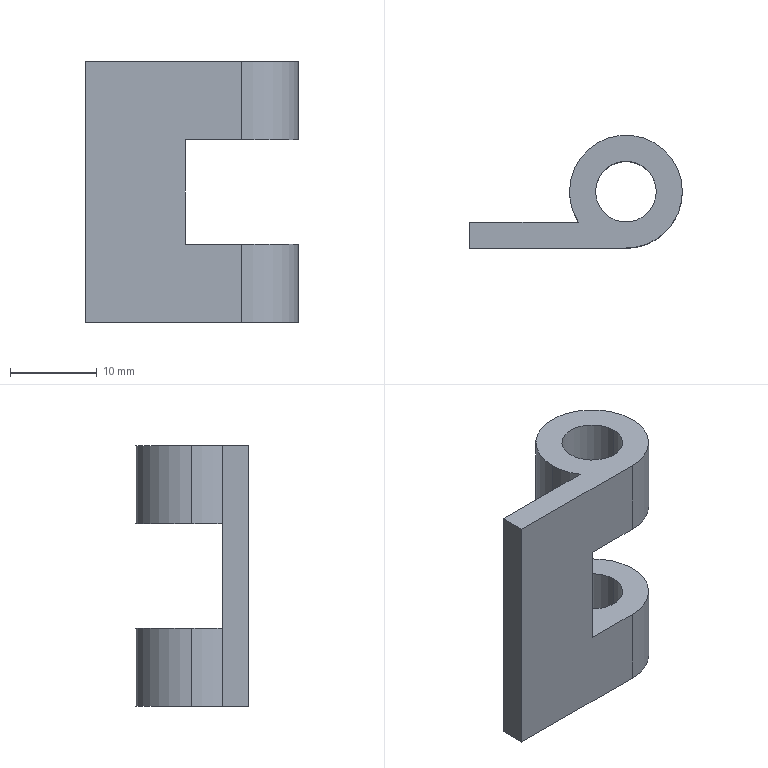Part | SolidWorks | features Extrusion 1, ICE 1 | 1 solid | 18 faces | box 24.5 x 13 x 30 mm | volume 2874 mm3 | cylinder 10 | plane 8 | commonest cylinder face diameters 13 x6 7 x4
STEP:
#1=CARTESIAN_POINT('',(5.5,5.,30.));
#2=VERTEX_POINT('',#1);
#3=CARTESIAN_POINT('',(12.5,5.,30.));
#4=VERTEX_POINT('',#3);
#5=CARTESIAN_POINT('',(9.,5.,30.));
#6=DIRECTION('',(0.,0.,1.));
#7=DIRECTION('',(1.,0.,0.));
#8=AXIS2_PLACEMENT_3D('',#5,#6,#7);
#9=CIRCLE('',#8,3.5);
#10=EDGE_CURVE('',#2,#4,#9,.T.);
#11=ORIENTED_EDGE('',*,*,#10,.T.);
#12=CARTESIAN_POINT('',(12.5,5.,21.));
#13=VERTEX_POINT('',#12);
#14=CARTESIAN_POINT('',(12.5,5.,30.));
#15=DIRECTION('',(0.,0.,-1.));
#16=VECTOR('',#15,1000.);
#17=LINE('',#14,#16);
#18=EDGE_CURVE('',#4,#13,#17,.T.);
#19=ORIENTED_EDGE('',*,*,#18,.T.);
#20=CARTESIAN_POINT('',(5.5,5.,21.));
#21=VERTEX_POINT('',#20);
#22=CARTESIAN_POINT('',(9.,5.,21.));
#23=DIRECTION('',(0.,0.,1.));
#24=DIRECTION('',(1.,0.,0.));
#25=AXIS2_PLACEMENT_3D('',#22,#23,#24);
#26=CIRCLE('',#25,3.5);
#27=EDGE_CURVE('',#21,#13,#26,.T.);
#28=ORIENTED_EDGE('',*,*,#27,.F.);
#29=CARTESIAN_POINT('',(5.5,5.,30.));
#30=DIRECTION('',(0.,0.,-1.));
#31=VECTOR('',#30,1000.);
#32=LINE('',#29,#31);
#33=EDGE_CURVE('',#2,#21,#32,.T.);
#34=ORIENTED_EDGE('',*,*,#33,.F.);
#35=EDGE_LOOP('',(#11,#19,#28,#34));
#36=FACE_OUTER_BOUND('',#35,.T.);
#37=CARTESIAN_POINT('',(9.,5.,30.));
#38=DIRECTION('',(0.,0.,-1.));
#39=DIRECTION('',(-1.,0.,0.));
#40=AXIS2_PLACEMENT_3D('',#37,#38,#39);
#41=CYLINDRICAL_SURFACE('',#40,3.5);
#42=ADVANCED_FACE('',(#36),#41,.F.);
#43=CARTESIAN_POINT('',(15.5,5.,30.));
#44=VERTEX_POINT('',#43);
#45=CARTESIAN_POINT('',(2.5,5.,30.));
#46=VERTEX_POINT('',#45);
#47=CARTESIAN_POINT('',(9.,5.,30.));
#48=DIRECTION('',(0.,0.,1.));
#49=DIRECTION('',(1.,0.,0.));
#50=AXIS2_PLACEMENT_3D('',#47,#48,#49);
#51=CIRCLE('',#50,6.5);
#52=EDGE_CURVE('',#44,#46,#51,.T.);
#53=ORIENTED_EDGE('',*,*,#52,.F.);
#54=CARTESIAN_POINT('',(15.5,5.,21.));
#55=VERTEX_POINT('',#54);
#56=CARTESIAN_POINT('',(15.5,5.,30.));
#57=DIRECTION('',(0.,0.,-1.));
#58=VECTOR('',#57,1000.);
#59=LINE('',#56,#58);
#60=EDGE_CURVE('',#44,#55,#59,.T.);
#61=ORIENTED_EDGE('',*,*,#60,.T.);
#62=CARTESIAN_POINT('',(2.5,5.,21.));
#63=VERTEX_POINT('',#62);
#64=CARTESIAN_POINT('',(9.,5.,21.));
#65=DIRECTION('',(0.,0.,1.));
#66=DIRECTION('',(1.,0.,0.));
#67=AXIS2_PLACEMENT_3D('',#64,#65,#66);
#68=CIRCLE('',#67,6.5);
#69=EDGE_CURVE('',#55,#63,#68,.T.);
#70=ORIENTED_EDGE('',*,*,#69,.T.);
#71=CARTESIAN_POINT('',(2.5,5.,30.));
#72=DIRECTION('',(0.,0.,-1.));
#73=VECTOR('',#72,1000.);
#74=LINE('',#71,#73);
#75=EDGE_CURVE('',#46,#63,#74,.T.);
#76=ORIENTED_EDGE('',*,*,#75,.F.);
#77=EDGE_LOOP('',(#53,#61,#70,#76));
#78=FACE_OUTER_BOUND('',#77,.T.);
#79=CARTESIAN_POINT('',(9.,5.,30.));
#80=DIRECTION('',(0.,0.,-1.));
#81=DIRECTION('',(-1.,0.,0.));
#82=AXIS2_PLACEMENT_3D('',#79,#80,#81);
#83=CYLINDRICAL_SURFACE('',#82,6.5);
#84=ADVANCED_FACE('',(#78),#83,.T.);
#85=CARTESIAN_POINT('',(3.523,1.5,30.));
#86=VERTEX_POINT('',#85);
#87=CARTESIAN_POINT('',(9.,5.,30.));
#88=DIRECTION('',(0.,0.,1.));
#89=DIRECTION('',(1.,0.,0.));
#90=AXIS2_PLACEMENT_3D('',#87,#88,#89);
#91=CIRCLE('',#90,6.5);
#92=EDGE_CURVE('',#46,#86,#91,.T.);
#93=ORIENTED_EDGE('',*,*,#92,.F.);
#94=ORIENTED_EDGE('',*,*,#75,.T.);
#95=CARTESIAN_POINT('',(3.523,1.5,21.));
#96=VERTEX_POINT('',#95);
#97=CARTESIAN_POINT('',(9.,5.,21.));
#98=DIRECTION('',(0.,0.,1.));
#99=DIRECTION('',(1.,0.,0.));
#100=AXIS2_PLACEMENT_3D('',#97,#98,#99);
#101=CIRCLE('',#100,6.5);
#102=EDGE_CURVE('',#63,#96,#101,.T.);
#103=ORIENTED_EDGE('',*,*,#102,.T.);
#104=CARTESIAN_POINT('',(3.523,1.5,30.));
#105=DIRECTION('',(0.,0.,-1.));
#106=VECTOR('',#105,1000.);
#107=LINE('',#104,#106);
#108=EDGE_CURVE('',#86,#96,#107,.T.);
#109=ORIENTED_EDGE('',*,*,#108,.F.);
#110=EDGE_LOOP('',(#93,#94,#103,#109));
#111=FACE_OUTER_BOUND('',#110,.T.);
#112=CARTESIAN_POINT('',(9.,5.,30.));
#113=DIRECTION('',(0.,0.,-1.));
#114=DIRECTION('',(-1.,0.,0.));
#115=AXIS2_PLACEMENT_3D('',#112,#113,#114);
#116=CYLINDRICAL_SURFACE('',#115,6.5);
#117=ADVANCED_FACE('',(#111),#116,.T.);
#118=CARTESIAN_POINT('',(12.5,5.,9.));
#119=VERTEX_POINT('',#118);
#120=CARTESIAN_POINT('',(5.5,5.,9.));
#121=VERTEX_POINT('',#120);
#122=CARTESIAN_POINT('',(9.,5.,9.));
#123=DIRECTION('',(0.,0.,-1.));
#124=DIRECTION('',(-1.,0.,0.));
#125=AXIS2_PLACEMENT_3D('',#122,#123,#124);
#126=CIRCLE('',#125,3.5);
#127=EDGE_CURVE('',#119,#121,#126,.T.);
#128=ORIENTED_EDGE('',*,*,#127,.F.);
#129=CARTESIAN_POINT('',(12.5,5.,0.));
#130=VERTEX_POINT('',#129);
#131=CARTESIAN_POINT('',(12.5,5.,30.));
#132=DIRECTION('',(0.,0.,-1.));
#133=VECTOR('',#132,1000.);
#134=LINE('',#131,#133);
#135=EDGE_CURVE('',#119,#130,#134,.T.);
#136=ORIENTED_EDGE('',*,*,#135,.T.);
#137=CARTESIAN_POINT('',(5.5,5.,0.));
#138=VERTEX_POINT('',#137);
#139=CARTESIAN_POINT('',(9.,5.,0.));
#140=DIRECTION('',(0.,0.,1.));
#141=DIRECTION('',(1.,0.,0.));
#142=AXIS2_PLACEMENT_3D('',#139,#140,#141);
#143=CIRCLE('',#142,3.5);
#144=EDGE_CURVE('',#138,#130,#143,.T.);
#145=ORIENTED_EDGE('',*,*,#144,.F.);
#146=CARTESIAN_POINT('',(5.5,5.,30.));
#147=DIRECTION('',(0.,0.,-1.));
#148=VECTOR('',#147,1000.);
#149=LINE('',#146,#148);
#150=EDGE_CURVE('',#121,#138,#149,.T.);
#151=ORIENTED_EDGE('',*,*,#150,.F.);
#152=EDGE_LOOP('',(#128,#136,#145,#151));
#153=FACE_OUTER_BOUND('',#152,.T.);
#154=CARTESIAN_POINT('',(9.,5.,30.));
#155=DIRECTION('',(0.,0.,-1.));
#156=DIRECTION('',(-1.,0.,0.));
#157=AXIS2_PLACEMENT_3D('',#154,#155,#156);
#158=CYLINDRICAL_SURFACE('',#157,3.5);
#159=ADVANCED_FACE('',(#153),#158,.F.);
#160=CARTESIAN_POINT('',(2.5,5.,9.));
#161=VERTEX_POINT('',#160);
#162=CARTESIAN_POINT('',(15.5,5.,9.));
#163=VERTEX_POINT('',#162);
#164=CARTESIAN_POINT('',(9.,5.,9.));
#165=DIRECTION('',(0.,0.,-1.));
#166=DIRECTION('',(-1.,0.,0.));
#167=AXIS2_PLACEMENT_3D('',#164,#165,#166);
#168=CIRCLE('',#167,6.5);
#169=EDGE_CURVE('',#161,#163,#168,.T.);
#170=ORIENTED_EDGE('',*,*,#169,.T.);
#171=CARTESIAN_POINT('',(15.5,5.,0.));
#172=VERTEX_POINT('',#171);
#173=CARTESIAN_POINT('',(15.5,5.,30.));
#174=DIRECTION('',(0.,0.,-1.));
#175=VECTOR('',#174,1000.);
#176=LINE('',#173,#175);
#177=EDGE_CURVE('',#163,#172,#176,.T.);
#178=ORIENTED_EDGE('',*,*,#177,.T.);
#179=CARTESIAN_POINT('',(2.5,5.,0.));
#180=VERTEX_POINT('',#179);
#181=CARTESIAN_POINT('',(9.,5.,0.));
#182=DIRECTION('',(0.,0.,1.));
#183=DIRECTION('',(1.,0.,0.));
#184=AXIS2_PLACEMENT_3D('',#181,#182,#183);
#185=CIRCLE('',#184,6.5);
#186=EDGE_CURVE('',#172,#180,#185,.T.);
#187=ORIENTED_EDGE('',*,*,#186,.T.);
#188=CARTESIAN_POINT('',(2.5,5.,30.));
#189=DIRECTION('',(0.,0.,-1.));
#190=VECTOR('',#189,1000.);
#191=LINE('',#188,#190);
#192=EDGE_CURVE('',#161,#180,#191,.T.);
#193=ORIENTED_EDGE('',*,*,#192,.F.);
#194=EDGE_LOOP('',(#170,#178,#187,#193));
#195=FACE_OUTER_BOUND('',#194,.T.);
#196=CARTESIAN_POINT('',(9.,5.,30.));
#197=DIRECTION('',(0.,0.,-1.));
#198=DIRECTION('',(-1.,0.,0.));
#199=AXIS2_PLACEMENT_3D('',#196,#197,#198);
#200=CYLINDRICAL_SURFACE('',#199,6.5);
#201=ADVANCED_FACE('',(#195),#200,.T.);
#202=CARTESIAN_POINT('',(3.523,1.5,9.));
#203=VERTEX_POINT('',#202);
#204=CARTESIAN_POINT('',(9.,5.,9.));
#205=DIRECTION('',(0.,0.,-1.));
#206=DIRECTION('',(-1.,0.,0.));
#207=AXIS2_PLACEMENT_3D('',#204,#205,#206);
#208=CIRCLE('',#207,6.5);
#209=EDGE_CURVE('',#203,#161,#208,.T.);
#210=ORIENTED_EDGE('',*,*,#209,.T.);
#211=ORIENTED_EDGE('',*,*,#192,.T.);
#212=CARTESIAN_POINT('',(3.523,1.5,0.));
#213=VERTEX_POINT('',#212);
#214=CARTESIAN_POINT('',(9.,5.,0.));
#215=DIRECTION('',(0.,0.,1.));
#216=DIRECTION('',(1.,0.,0.));
#217=AXIS2_PLACEMENT_3D('',#214,#215,#216);
#218=CIRCLE('',#217,6.5);
#219=EDGE_CURVE('',#180,#213,#218,.T.);
#220=ORIENTED_EDGE('',*,*,#219,.T.);
#221=CARTESIAN_POINT('',(3.523,1.5,30.));
#222=DIRECTION('',(0.,0.,-1.));
#223=VECTOR('',#222,1000.);
#224=LINE('',#221,#223);
#225=EDGE_CURVE('',#203,#213,#224,.T.);
#226=ORIENTED_EDGE('',*,*,#225,.F.);
#227=EDGE_LOOP('',(#210,#211,#220,#226));
#228=FACE_OUTER_BOUND('',#227,.T.);
#229=CARTESIAN_POINT('',(9.,5.,30.));
#230=DIRECTION('',(0.,0.,-1.));
#231=DIRECTION('',(-1.,0.,0.));
#232=AXIS2_PLACEMENT_3D('',#229,#230,#231);
#233=CYLINDRICAL_SURFACE('',#232,6.5);
#234=ADVANCED_FACE('',(#228),#233,.T.);
#235=ORIENTED_EDGE('',*,*,#177,.F.);
#236=CARTESIAN_POINT('',(9.,-1.5,9.));
#237=VERTEX_POINT('',#236);
#238=CARTESIAN_POINT('',(9.,5.,9.));
#239=DIRECTION('',(0.,0.,-1.));
#240=DIRECTION('',(-1.,0.,0.));
#241=AXIS2_PLACEMENT_3D('',#238,#239,#240);
#242=CIRCLE('',#241,6.5);
#243=EDGE_CURVE('',#163,#237,#242,.T.);
#244=ORIENTED_EDGE('',*,*,#243,.T.);
#245=CARTESIAN_POINT('',(9.,-1.5,0.));
#246=VERTEX_POINT('',#245);
#247=CARTESIAN_POINT('',(9.,-1.5,30.));
#248=DIRECTION('',(0.,0.,-1.));
#249=VECTOR('',#248,1000.);
#250=LINE('',#247,#249);
#251=EDGE_CURVE('',#237,#246,#250,.T.);
#252=ORIENTED_EDGE('',*,*,#251,.T.);
#253=CARTESIAN_POINT('',(9.,5.,0.));
#254=DIRECTION('',(0.,0.,1.));
#255=DIRECTION('',(1.,0.,0.));
#256=AXIS2_PLACEMENT_3D('',#253,#254,#255);
#257=CIRCLE('',#256,6.5);
#258=EDGE_CURVE('',#246,#172,#257,.T.);
#259=ORIENTED_EDGE('',*,*,#258,.T.);
#260=EDGE_LOOP('',(#235,#244,#252,#259));
#261=FACE_OUTER_BOUND('',#260,.T.);
#262=CARTESIAN_POINT('',(9.,5.,30.));
#263=DIRECTION('',(0.,0.,-1.));
#264=DIRECTION('',(-1.,0.,0.));
#265=AXIS2_PLACEMENT_3D('',#262,#263,#264);
#266=CYLINDRICAL_SURFACE('',#265,6.5);
#267=ADVANCED_FACE('',(#261),#266,.T.);
#268=ORIENTED_EDGE('',*,*,#135,.F.);
#269=CARTESIAN_POINT('',(9.,5.,9.));
#270=DIRECTION('',(0.,0.,-1.));
#271=DIRECTION('',(-1.,0.,0.));
#272=AXIS2_PLACEMENT_3D('',#269,#270,#271);
#273=CIRCLE('',#272,3.5);
#274=EDGE_CURVE('',#121,#119,#273,.T.);
#275=ORIENTED_EDGE('',*,*,#274,.F.);
#276=ORIENTED_EDGE('',*,*,#150,.T.);
#277=CARTESIAN_POINT('',(9.,5.,0.));
#278=DIRECTION('',(0.,0.,1.));
#279=DIRECTION('',(1.,0.,0.));
#280=AXIS2_PLACEMENT_3D('',#277,#278,#279);
#281=CIRCLE('',#280,3.5);
#282=EDGE_CURVE('',#130,#138,#281,.T.);
#283=ORIENTED_EDGE('',*,*,#282,.F.);
#284=EDGE_LOOP('',(#268,#275,#276,#283));
#285=FACE_OUTER_BOUND('',#284,.T.);
#286=CARTESIAN_POINT('',(9.,5.,30.));
#287=DIRECTION('',(0.,0.,-1.));
#288=DIRECTION('',(-1.,0.,0.));
#289=AXIS2_PLACEMENT_3D('',#286,#287,#288);
#290=CYLINDRICAL_SURFACE('',#289,3.5);
#291=ADVANCED_FACE('',(#285),#290,.F.);
#292=CARTESIAN_POINT('',(9.,-1.5,30.));
#293=VERTEX_POINT('',#292);
#294=CARTESIAN_POINT('',(9.,5.,30.));
#295=DIRECTION('',(0.,0.,1.));
#296=DIRECTION('',(1.,0.,0.));
#297=AXIS2_PLACEMENT_3D('',#294,#295,#296);
#298=CIRCLE('',#297,6.5);
#299=EDGE_CURVE('',#293,#44,#298,.T.);
#300=ORIENTED_EDGE('',*,*,#299,.T.);
#301=ORIENTED_EDGE('',*,*,#52,.T.);
#302=ORIENTED_EDGE('',*,*,#92,.T.);
#303=CARTESIAN_POINT('',(-9.,1.5,30.));
#304=VERTEX_POINT('',#303);
#305=CARTESIAN_POINT('',(-9.,1.5,30.));
#306=DIRECTION('',(-1.,0.,0.));
#307=VECTOR('',#306,1000.);
#308=LINE('',#305,#307);
#309=EDGE_CURVE('',#86,#304,#308,.T.);
#310=ORIENTED_EDGE('',*,*,#309,.T.);
#311=CARTESIAN_POINT('',(-9.,-1.5,30.));
#312=VERTEX_POINT('',#311);
#313=CARTESIAN_POINT('',(-9.,1.5,30.));
#314=DIRECTION('',(0.,-1.,0.));
#315=VECTOR('',#314,1000.);
#316=LINE('',#313,#315);
#317=EDGE_CURVE('',#304,#312,#316,.T.);
#318=ORIENTED_EDGE('',*,*,#317,.T.);
#319=CARTESIAN_POINT('',(-9.,-1.5,30.));
#320=DIRECTION('',(1.,0.,0.));
#321=VECTOR('',#320,1000.);
#322=LINE('',#319,#321);
#323=EDGE_CURVE('',#312,#293,#322,.T.);
#324=ORIENTED_EDGE('',*,*,#323,.T.);
#325=EDGE_LOOP('',(#300,#301,#302,#310,#318,#324));
#326=FACE_OUTER_BOUND('',#325,.T.);
#327=ORIENTED_EDGE('',*,*,#10,.F.);
#328=CARTESIAN_POINT('',(9.,5.,30.));
#329=DIRECTION('',(0.,0.,1.));
#330=DIRECTION('',(1.,0.,0.));
#331=AXIS2_PLACEMENT_3D('',#328,#329,#330);
#332=CIRCLE('',#331,3.5);
#333=EDGE_CURVE('',#4,#2,#332,.T.);
#334=ORIENTED_EDGE('',*,*,#333,.F.);
#335=EDGE_LOOP('',(#327,#334));
#336=FACE_BOUND('',#335,.T.);
#337=CARTESIAN_POINT('',(9.,5.,30.));
#338=DIRECTION('',(0.,0.,1.));
#339=DIRECTION('',(1.,0.,0.));
#340=AXIS2_PLACEMENT_3D('',#337,#338,#339);
#341=PLANE('',#340);
#342=ADVANCED_FACE('',(#326,#336),#341,.T.);
#343=ORIENTED_EDGE('',*,*,#258,.F.);
#344=CARTESIAN_POINT('',(-9.,-1.5,0.));
#345=VERTEX_POINT('',#344);
#346=CARTESIAN_POINT('',(-9.,-1.5,0.));
#347=DIRECTION('',(1.,0.,0.));
#348=VECTOR('',#347,1000.);
#349=LINE('',#346,#348);
#350=EDGE_CURVE('',#345,#246,#349,.T.);
#351=ORIENTED_EDGE('',*,*,#350,.F.);
#352=CARTESIAN_POINT('',(-9.,1.5,0.));
#353=VERTEX_POINT('',#352);
#354=CARTESIAN_POINT('',(-9.,1.5,0.));
#355=DIRECTION('',(0.,-1.,0.));
#356=VECTOR('',#355,1000.);
#357=LINE('',#354,#356);
#358=EDGE_CURVE('',#353,#345,#357,.T.);
#359=ORIENTED_EDGE('',*,*,#358,.F.);
#360=CARTESIAN_POINT('',(-9.,1.5,0.));
#361=DIRECTION('',(-1.,0.,0.));
#362=VECTOR('',#361,1000.);
#363=LINE('',#360,#362);
#364=EDGE_CURVE('',#213,#353,#363,.T.);
#365=ORIENTED_EDGE('',*,*,#364,.F.);
#366=ORIENTED_EDGE('',*,*,#219,.F.);
#367=ORIENTED_EDGE('',*,*,#186,.F.);
#368=EDGE_LOOP('',(#343,#351,#359,#365,#366,#367));
#369=FACE_OUTER_BOUND('',#368,.T.);
#370=ORIENTED_EDGE('',*,*,#144,.T.);
#371=ORIENTED_EDGE('',*,*,#282,.T.);
#372=EDGE_LOOP('',(#370,#371));
#373=FACE_BOUND('',#372,.T.);
#374=CARTESIAN_POINT('',(9.,5.,0.));
#375=DIRECTION('',(0.,0.,1.));
#376=DIRECTION('',(1.,0.,0.));
#377=AXIS2_PLACEMENT_3D('',#374,#375,#376);
#378=PLANE('',#377);
#379=ADVANCED_FACE('',(#369,#373),#378,.F.);
#380=ORIENTED_EDGE('',*,*,#60,.F.);
#381=ORIENTED_EDGE('',*,*,#299,.F.);
#382=CARTESIAN_POINT('',(9.,-1.5,21.));
#383=VERTEX_POINT('',#382);
#384=CARTESIAN_POINT('',(9.,-1.5,30.));
#385=DIRECTION('',(0.,0.,-1.));
#386=VECTOR('',#385,1000.);
#387=LINE('',#384,#386);
#388=EDGE_CURVE('',#293,#383,#387,.T.);
#389=ORIENTED_EDGE('',*,*,#388,.T.);
#390=CARTESIAN_POINT('',(9.,5.,21.));
#391=DIRECTION('',(0.,0.,1.));
#392=DIRECTION('',(1.,0.,0.));
#393=AXIS2_PLACEMENT_3D('',#390,#391,#392);
#394=CIRCLE('',#393,6.5);
#395=EDGE_CURVE('',#383,#55,#394,.T.);
#396=ORIENTED_EDGE('',*,*,#395,.T.);
#397=EDGE_LOOP('',(#380,#381,#389,#396));
#398=FACE_OUTER_BOUND('',#397,.T.);
#399=CARTESIAN_POINT('',(9.,5.,30.));
#400=DIRECTION('',(0.,0.,-1.));
#401=DIRECTION('',(-1.,0.,0.));
#402=AXIS2_PLACEMENT_3D('',#399,#400,#401);
#403=CYLINDRICAL_SURFACE('',#402,6.5);
#404=ADVANCED_FACE('',(#398),#403,.T.);
#405=CARTESIAN_POINT('',(2.5,1.5,21.));
#406=VERTEX_POINT('',#405);
#407=CARTESIAN_POINT('',(2.5,1.5,9.));
#408=VERTEX_POINT('',#407);
#409=CARTESIAN_POINT('',(2.5,1.5,30.));
#410=DIRECTION('',(0.,0.,-1.));
#411=VECTOR('',#410,1000.);
#412=LINE('',#409,#411);
#413=EDGE_CURVE('',#406,#408,#412,.T.);
#414=ORIENTED_EDGE('',*,*,#413,.T.);
#415=CARTESIAN_POINT('',(-9.,1.5,9.));
#416=DIRECTION('',(1.,0.,0.));
#417=VECTOR('',#416,1000.);
#418=LINE('',#415,#417);
#419=EDGE_CURVE('',#408,#203,#418,.T.);
#420=ORIENTED_EDGE('',*,*,#419,.T.);
#421=ORIENTED_EDGE('',*,*,#225,.T.);
#422=ORIENTED_EDGE('',*,*,#364,.T.);
#423=CARTESIAN_POINT('',(-9.,1.5,30.));
#424=DIRECTION('',(0.,0.,-1.));
#425=VECTOR('',#424,1000.);
#426=LINE('',#423,#425);
#427=EDGE_CURVE('',#304,#353,#426,.T.);
#428=ORIENTED_EDGE('',*,*,#427,.F.);
#429=ORIENTED_EDGE('',*,*,#309,.F.);
#430=ORIENTED_EDGE('',*,*,#108,.T.);
#431=CARTESIAN_POINT('',(-9.,1.5,21.));
#432=DIRECTION('',(-1.,0.,0.));
#433=VECTOR('',#432,1000.);
#434=LINE('',#431,#433);
#435=EDGE_CURVE('',#96,#406,#434,.T.);
#436=ORIENTED_EDGE('',*,*,#435,.T.);
#437=EDGE_LOOP('',(#414,#420,#421,#422,#428,#429,#430,#436));
#438=FACE_OUTER_BOUND('',#437,.T.);
#439=CARTESIAN_POINT('',(-9.,1.5,30.));
#440=DIRECTION('',(0.,-1.,0.));
#441=DIRECTION('',(0.,0.,-1.));
#442=AXIS2_PLACEMENT_3D('',#439,#440,#441);
#443=PLANE('',#442);
#444=ADVANCED_FACE('',(#438),#443,.F.);
#445=ORIENTED_EDGE('',*,*,#358,.T.);
#446=CARTESIAN_POINT('',(-9.,-1.5,30.));
#447=DIRECTION('',(0.,0.,-1.));
#448=VECTOR('',#447,1000.);
#449=LINE('',#446,#448);
#450=EDGE_CURVE('',#312,#345,#449,.T.);
#451=ORIENTED_EDGE('',*,*,#450,.F.);
#452=ORIENTED_EDGE('',*,*,#317,.F.);
#453=ORIENTED_EDGE('',*,*,#427,.T.);
#454=EDGE_LOOP('',(#445,#451,#452,#453));
#455=FACE_OUTER_BOUND('',#454,.T.);
#456=CARTESIAN_POINT('',(-9.,1.5,30.));
#457=DIRECTION('',(1.,0.,0.));
#458=DIRECTION('',(0.,0.,-1.));
#459=AXIS2_PLACEMENT_3D('',#456,#457,#458);
#460=PLANE('',#459);
#461=ADVANCED_FACE('',(#455),#460,.F.);
#462=ORIENTED_EDGE('',*,*,#251,.F.);
#463=CARTESIAN_POINT('',(2.5,-1.5,9.));
#464=VERTEX_POINT('',#463);
#465=CARTESIAN_POINT('',(-9.,-1.5,9.));
#466=DIRECTION('',(-1.,0.,0.));
#467=VECTOR('',#466,1000.);
#468=LINE('',#465,#467);
#469=EDGE_CURVE('',#237,#464,#468,.T.);
#470=ORIENTED_EDGE('',*,*,#469,.T.);
#471=CARTESIAN_POINT('',(2.5,-1.5,21.));
#472=VERTEX_POINT('',#471);
#473=CARTESIAN_POINT('',(2.5,-1.5,30.));
#474=DIRECTION('',(0.,0.,1.));
#475=VECTOR('',#474,1000.);
#476=LINE('',#473,#475);
#477=EDGE_CURVE('',#464,#472,#476,.T.);
#478=ORIENTED_EDGE('',*,*,#477,.T.);
#479=CARTESIAN_POINT('',(-9.,-1.5,21.));
#480=DIRECTION('',(1.,0.,0.));
#481=VECTOR('',#480,1000.);
#482=LINE('',#479,#481);
#483=EDGE_CURVE('',#472,#383,#482,.T.);
#484=ORIENTED_EDGE('',*,*,#483,.T.);
#485=ORIENTED_EDGE('',*,*,#388,.F.);
#486=ORIENTED_EDGE('',*,*,#323,.F.);
#487=ORIENTED_EDGE('',*,*,#450,.T.);
#488=ORIENTED_EDGE('',*,*,#350,.T.);
#489=EDGE_LOOP('',(#462,#470,#478,#484,#485,#486,#487,#488));
#490=FACE_OUTER_BOUND('',#489,.T.);
#491=CARTESIAN_POINT('',(-9.,-1.5,30.));
#492=DIRECTION('',(0.,1.,0.));
#493=DIRECTION('',(0.,0.,1.));
#494=AXIS2_PLACEMENT_3D('',#491,#492,#493);
#495=PLANE('',#494);
#496=ADVANCED_FACE('',(#490),#495,.F.);
#497=ORIENTED_EDGE('',*,*,#18,.F.);
#498=ORIENTED_EDGE('',*,*,#333,.T.);
#499=ORIENTED_EDGE('',*,*,#33,.T.);
#500=CARTESIAN_POINT('',(9.,5.,21.));
#501=DIRECTION('',(0.,0.,1.));
#502=DIRECTION('',(1.,0.,0.));
#503=AXIS2_PLACEMENT_3D('',#500,#501,#502);
#504=CIRCLE('',#503,3.5);
#505=EDGE_CURVE('',#13,#21,#504,.T.);
#506=ORIENTED_EDGE('',*,*,#505,.F.);
#507=EDGE_LOOP('',(#497,#498,#499,#506));
#508=FACE_OUTER_BOUND('',#507,.T.);
#509=CARTESIAN_POINT('',(9.,5.,30.));
#510=DIRECTION('',(0.,0.,-1.));
#511=DIRECTION('',(-1.,0.,0.));
#512=AXIS2_PLACEMENT_3D('',#509,#510,#511);
#513=CYLINDRICAL_SURFACE('',#512,3.5);
#514=ADVANCED_FACE('',(#508),#513,.F.);
#515=CARTESIAN_POINT('',(2.5,-15.,21.));
#516=DIRECTION('',(0.,1.,0.));
#517=VECTOR('',#516,1000.);
#518=LINE('',#515,#517);
#519=EDGE_CURVE('',#472,#406,#518,.T.);
#520=ORIENTED_EDGE('',*,*,#519,.F.);
#521=ORIENTED_EDGE('',*,*,#477,.F.);
#522=CARTESIAN_POINT('',(2.5,-15.,9.));
#523=DIRECTION('',(0.,1.,0.));
#524=VECTOR('',#523,1000.);
#525=LINE('',#522,#524);
#526=EDGE_CURVE('',#464,#408,#525,.T.);
#527=ORIENTED_EDGE('',*,*,#526,.T.);
#528=ORIENTED_EDGE('',*,*,#413,.F.);
#529=EDGE_LOOP('',(#520,#521,#527,#528));
#530=FACE_OUTER_BOUND('',#529,.T.);
#531=CARTESIAN_POINT('',(2.5,-15.,9.));
#532=DIRECTION('',(-1.,0.,0.));
#533=DIRECTION('',(0.,0.,1.));
#534=AXIS2_PLACEMENT_3D('',#531,#532,#533);
#535=PLANE('',#534);
#536=ADVANCED_FACE('',(#530),#535,.F.);
#537=ORIENTED_EDGE('',*,*,#274,.T.);
#538=ORIENTED_EDGE('',*,*,#127,.T.);
#539=EDGE_LOOP('',(#537,#538));
#540=FACE_BOUND('',#539,.T.);
#541=ORIENTED_EDGE('',*,*,#526,.F.);
#542=ORIENTED_EDGE('',*,*,#469,.F.);
#543=ORIENTED_EDGE('',*,*,#243,.F.);
#544=ORIENTED_EDGE('',*,*,#169,.F.);
#545=ORIENTED_EDGE('',*,*,#209,.F.);
#546=ORIENTED_EDGE('',*,*,#419,.F.);
#547=EDGE_LOOP('',(#541,#542,#543,#544,#545,#546));
#548=FACE_OUTER_BOUND('',#547,.T.);
#549=CARTESIAN_POINT('',(2.5,-15.,9.));
#550=DIRECTION('',(0.,0.,-1.));
#551=DIRECTION('',(-1.,0.,0.));
#552=AXIS2_PLACEMENT_3D('',#549,#550,#551);
#553=PLANE('',#552);
#554=ADVANCED_FACE('',(#540,#548),#553,.F.);
#555=ORIENTED_EDGE('',*,*,#27,.T.);
#556=ORIENTED_EDGE('',*,*,#505,.T.);
#557=EDGE_LOOP('',(#555,#556));
#558=FACE_BOUND('',#557,.T.);
#559=ORIENTED_EDGE('',*,*,#395,.F.);
#560=ORIENTED_EDGE('',*,*,#483,.F.);
#561=ORIENTED_EDGE('',*,*,#519,.T.);
#562=ORIENTED_EDGE('',*,*,#435,.F.);
#563=ORIENTED_EDGE('',*,*,#102,.F.);
#564=ORIENTED_EDGE('',*,*,#69,.F.);
#565=EDGE_LOOP('',(#559,#560,#561,#562,#563,#564));
#566=FACE_OUTER_BOUND('',#565,.T.);
#567=CARTESIAN_POINT('',(2.5,-15.,21.));
#568=DIRECTION('',(0.,0.,1.));
#569=DIRECTION('',(1.,0.,0.));
#570=AXIS2_PLACEMENT_3D('',#567,#568,#569);
#571=PLANE('',#570);
#572=ADVANCED_FACE('',(#558,#566),#571,.F.);
#573=CLOSED_SHELL('',(#42,#84,#117,#159,#201,#234,#267,#291,#342,#379,#404,#444,#461,#496,#514,#536,#554,#572));
#574=MANIFOLD_SOLID_BREP('',#573);
#575=CARTESIAN_POINT('',(0.,0.,0.));
#576=DIRECTION('',(0.,0.,1.));
#577=DIRECTION('',(1.,0.,0.));
#578=AXIS2_PLACEMENT_3D('',#575,#576,#577);
#579=(LENGTH_UNIT()NAMED_UNIT(*)SI_UNIT(.MILLI.,.METRE.));
#580=UNCERTAINTY_MEASURE_WITH_UNIT(LENGTH_MEASURE(0.00001),#579,'','');
#581=(NAMED_UNIT(*)PLANE_ANGLE_UNIT()SI_UNIT($,.RADIAN.));
#582=(NAMED_UNIT(*)SI_UNIT($,.STERADIAN.)SOLID_ANGLE_UNIT());
#583=(GEOMETRIC_REPRESENTATION_CONTEXT(3)GLOBAL_UNCERTAINTY_ASSIGNED_CONTEXT((#580))GLOBAL_UNIT_ASSIGNED_CONTEXT((#579,#581,#582))REPRESENTATION_CONTEXT('',''));
#584=ADVANCED_BREP_SHAPE_REPRESENTATION('',(#574,#578),#583);